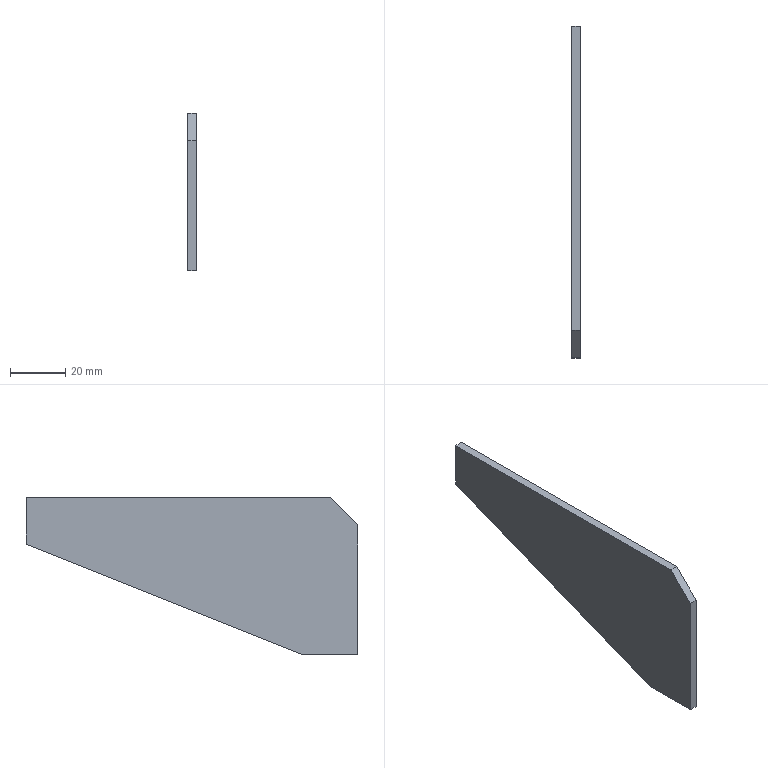Part | STEP file | HL4GZ-1.581.104 (tank support seat rib) | 1 solid | 8 faces | box 3 x 120 x 57 mm | volume 14370 mm3 | plane 8
STEP:
#1=CARTESIAN_POINT('',(0.,0.,0.));
#2=DIRECTION('',(0.,0.,1.));
#3=DIRECTION('',(1.,0.,0.));
#4=AXIS2_PLACEMENT_3D('',#1,#2,#3);
#5=CARTESIAN_POINT('',(1865.,-520.,-328.));
#6=VERTEX_POINT('',#5);
#7=CARTESIAN_POINT('',(1865.,-530.,-338.));
#8=VERTEX_POINT('',#7);
#9=CARTESIAN_POINT('',(1865.,-585.,-393.));
#10=DIRECTION('',(0.,-0.7071,-0.7071));
#11=VECTOR('',#10,1.);
#12=LINE('',#9,#11);
#13=CARTESIAN_POINT('',(1862.,-530.,-338.));
#14=DIRECTION('',(0.,0.7071,-0.7071));
#15=DIRECTION('',(1.,0.,0.));
#16=AXIS2_PLACEMENT_3D('',#13,#14,#15);
#17=PLANE('',#16);
#18=CARTESIAN_POINT('',(3.,77.782));
#19=DIRECTION('',(0.,1.));
#20=VECTOR('',#19,1.);
#21=LINE('',#18,#20);
#22=(GEOMETRIC_REPRESENTATION_CONTEXT(2)PARAMETRIC_REPRESENTATION_CONTEXT()REPRESENTATION_CONTEXT('',''));
#23=DEFINITIONAL_REPRESENTATION('',(#21),#22);
#24=PCURVE('',#17,#23);
#25=CARTESIAN_POINT('',(1865.,-653.,-325.));
#26=DIRECTION('',(1.,0.,0.));
#27=DIRECTION('',(0.,1.,0.));
#28=AXIS2_PLACEMENT_3D('',#25,#26,#27);
#29=PLANE('',#28);
#30=CARTESIAN_POINT('',(68.,-68.));
#31=DIRECTION('',(-0.7071,-0.7071));
#32=VECTOR('',#31,1.);
#33=LINE('',#30,#32);
#34=(GEOMETRIC_REPRESENTATION_CONTEXT(2)PARAMETRIC_REPRESENTATION_CONTEXT()REPRESENTATION_CONTEXT('',''));
#35=DEFINITIONAL_REPRESENTATION('',(#33),#34);
#36=PCURVE('',#29,#35);
#37=SURFACE_CURVE('',#12,(#24,#36),.PCURVE_S1.);
#38=EDGE_CURVE('',#6,#8,#37,.T.);
#39=ORIENTED_EDGE('',*,*,#38,.F.);
#40=CARTESIAN_POINT('',(1862.,-520.,-328.));
#41=VERTEX_POINT('',#40);
#42=CARTESIAN_POINT('',(1863.5,-520.,-328.));
#43=DIRECTION('',(1.,0.,0.));
#44=VECTOR('',#43,1.);
#45=LINE('',#42,#44);
#46=CARTESIAN_POINT('',(1.5,-14.142));
#47=DIRECTION('',(1.,0.));
#48=VECTOR('',#47,1.);
#49=LINE('',#46,#48);
#50=(GEOMETRIC_REPRESENTATION_CONTEXT(2)PARAMETRIC_REPRESENTATION_CONTEXT()REPRESENTATION_CONTEXT('',''));
#51=DEFINITIONAL_REPRESENTATION('',(#49),#50);
#52=PCURVE('',#17,#51);
#53=CARTESIAN_POINT('',(1863.5,-480.,-328.));
#54=DIRECTION('',(0.,0.,1.));
#55=DIRECTION('',(-1.,0.,0.));
#56=AXIS2_PLACEMENT_3D('',#53,#54,#55);
#57=PLANE('',#56);
#58=CARTESIAN_POINT('',(0.,40.));
#59=DIRECTION('',(-1.,0.));
#60=VECTOR('',#59,1.);
#61=LINE('',#58,#60);
#62=(GEOMETRIC_REPRESENTATION_CONTEXT(2)PARAMETRIC_REPRESENTATION_CONTEXT()REPRESENTATION_CONTEXT('',''));
#63=DEFINITIONAL_REPRESENTATION('',(#61),#62);
#64=PCURVE('',#57,#63);
#65=SURFACE_CURVE('',#45,(#52,#64),.PCURVE_S1.);
#66=EDGE_CURVE('',#41,#6,#65,.T.);
#67=ORIENTED_EDGE('',*,*,#66,.F.);
#68=CARTESIAN_POINT('',(1862.,-530.,-338.));
#69=VERTEX_POINT('',#68);
#70=CARTESIAN_POINT('',(1862.,-530.,-338.));
#71=DIRECTION('',(0.,0.7071,0.7071));
#72=VECTOR('',#71,1.);
#73=LINE('',#70,#72);
#74=CARTESIAN_POINT('',(0.,0.));
#75=DIRECTION('',(0.,-1.));
#76=VECTOR('',#75,1.);
#77=LINE('',#74,#76);
#78=(GEOMETRIC_REPRESENTATION_CONTEXT(2)PARAMETRIC_REPRESENTATION_CONTEXT()REPRESENTATION_CONTEXT('',''));
#79=DEFINITIONAL_REPRESENTATION('',(#77),#78);
#80=PCURVE('',#17,#79);
#81=CARTESIAN_POINT('',(1862.,-653.,-325.));
#82=DIRECTION('',(1.,0.,0.));
#83=DIRECTION('',(0.,1.,0.));
#84=AXIS2_PLACEMENT_3D('',#81,#82,#83);
#85=PLANE('',#84);
#86=CARTESIAN_POINT('',(123.,-13.));
#87=DIRECTION('',(0.7071,0.7071));
#88=VECTOR('',#87,1.);
#89=LINE('',#86,#88);
#90=(GEOMETRIC_REPRESENTATION_CONTEXT(2)PARAMETRIC_REPRESENTATION_CONTEXT()REPRESENTATION_CONTEXT('',''));
#91=DEFINITIONAL_REPRESENTATION('',(#89),#90);
#92=PCURVE('',#85,#91);
#93=SURFACE_CURVE('',#73,(#80,#92),.PCURVE_S1.);
#94=EDGE_CURVE('',#69,#41,#93,.T.);
#95=ORIENTED_EDGE('',*,*,#94,.F.);
#96=CARTESIAN_POINT('',(1862.,-530.,-338.));
#97=DIRECTION('',(-1.,0.,0.));
#98=VECTOR('',#97,1.);
#99=LINE('',#96,#98);
#100=CARTESIAN_POINT('',(0.,0.));
#101=DIRECTION('',(-1.,0.));
#102=VECTOR('',#101,1.);
#103=LINE('',#100,#102);
#104=(GEOMETRIC_REPRESENTATION_CONTEXT(2)PARAMETRIC_REPRESENTATION_CONTEXT()REPRESENTATION_CONTEXT('',''));
#105=DEFINITIONAL_REPRESENTATION('',(#103),#104);
#106=PCURVE('',#17,#105);
#107=CARTESIAN_POINT('',(1862.,-530.,-325.));
#108=DIRECTION('',(0.,-1.,0.));
#109=DIRECTION('',(0.,0.,1.));
#110=AXIS2_PLACEMENT_3D('',#107,#108,#109);
#111=PLANE('',#110);
#112=CARTESIAN_POINT('',(-13.,0.));
#113=DIRECTION('',(0.,1.));
#114=VECTOR('',#113,1.);
#115=LINE('',#112,#114);
#116=(GEOMETRIC_REPRESENTATION_CONTEXT(2)PARAMETRIC_REPRESENTATION_CONTEXT()REPRESENTATION_CONTEXT('',''));
#117=DEFINITIONAL_REPRESENTATION('',(#115),#116);
#118=PCURVE('',#111,#117);
#119=SURFACE_CURVE('',#99,(#106,#118),.PCURVE_S1.);
#120=EDGE_CURVE('',#8,#69,#119,.T.);
#121=ORIENTED_EDGE('',*,*,#120,.F.);
#122=EDGE_LOOP('',(#39,#67,#95,#121));
#123=FACE_BOUND('',#122,.T.);
#124=ADVANCED_FACE('',(#123),#17,.F.);
#125=CARTESIAN_POINT('',(1862.,-410.,-328.));
#126=VERTEX_POINT('',#125);
#127=CARTESIAN_POINT('',(1862.,-653.,-328.));
#128=DIRECTION('',(0.,-1.,0.));
#129=VECTOR('',#128,1.);
#130=LINE('',#127,#129);
#131=CARTESIAN_POINT('',(1.5,173.));
#132=DIRECTION('',(0.,1.));
#133=VECTOR('',#132,1.);
#134=LINE('',#131,#133);
#135=(GEOMETRIC_REPRESENTATION_CONTEXT(2)PARAMETRIC_REPRESENTATION_CONTEXT()REPRESENTATION_CONTEXT('',''));
#136=DEFINITIONAL_REPRESENTATION('',(#134),#135);
#137=PCURVE('',#57,#136);
#138=CARTESIAN_POINT('',(0.,-3.));
#139=DIRECTION('',(-1.,0.));
#140=VECTOR('',#139,1.);
#141=LINE('',#138,#140);
#142=(GEOMETRIC_REPRESENTATION_CONTEXT(2)PARAMETRIC_REPRESENTATION_CONTEXT()REPRESENTATION_CONTEXT('',''));
#143=DEFINITIONAL_REPRESENTATION('',(#141),#142);
#144=PCURVE('',#85,#143);
#145=SURFACE_CURVE('',#130,(#137,#144),.PCURVE_S1.);
#146=EDGE_CURVE('',#126,#41,#145,.T.);
#147=ORIENTED_EDGE('',*,*,#146,.T.);
#148=ORIENTED_EDGE('',*,*,#66,.T.);
#149=CARTESIAN_POINT('',(1865.,-410.,-328.));
#150=VERTEX_POINT('',#149);
#151=CARTESIAN_POINT('',(1865.,-653.,-328.));
#152=DIRECTION('',(0.,-1.,0.));
#153=VECTOR('',#152,1.);
#154=LINE('',#151,#153);
#155=CARTESIAN_POINT('',(-1.5,173.));
#156=DIRECTION('',(0.,1.));
#157=VECTOR('',#156,1.);
#158=LINE('',#155,#157);
#159=(GEOMETRIC_REPRESENTATION_CONTEXT(2)PARAMETRIC_REPRESENTATION_CONTEXT()REPRESENTATION_CONTEXT('',''));
#160=DEFINITIONAL_REPRESENTATION('',(#158),#159);
#161=PCURVE('',#57,#160);
#162=CARTESIAN_POINT('',(0.,-3.));
#163=DIRECTION('',(-1.,0.));
#164=VECTOR('',#163,1.);
#165=LINE('',#162,#164);
#166=(GEOMETRIC_REPRESENTATION_CONTEXT(2)PARAMETRIC_REPRESENTATION_CONTEXT()REPRESENTATION_CONTEXT('',''));
#167=DEFINITIONAL_REPRESENTATION('',(#165),#166);
#168=PCURVE('',#29,#167);
#169=SURFACE_CURVE('',#154,(#161,#168),.PCURVE_S1.);
#170=EDGE_CURVE('',#150,#6,#169,.T.);
#171=ORIENTED_EDGE('',*,*,#170,.F.);
#172=CARTESIAN_POINT('',(1862.,-410.,-328.));
#173=DIRECTION('',(1.,0.,0.));
#174=VECTOR('',#173,1.);
#175=LINE('',#172,#174);
#176=CARTESIAN_POINT('',(1.5,-70.));
#177=DIRECTION('',(-1.,0.));
#178=VECTOR('',#177,1.);
#179=LINE('',#176,#178);
#180=(GEOMETRIC_REPRESENTATION_CONTEXT(2)PARAMETRIC_REPRESENTATION_CONTEXT()REPRESENTATION_CONTEXT('',''));
#181=DEFINITIONAL_REPRESENTATION('',(#179),#180);
#182=PCURVE('',#57,#181);
#183=CARTESIAN_POINT('',(1862.,-410.,-325.));
#184=DIRECTION('',(0.,-1.,0.));
#185=DIRECTION('',(0.,0.,1.));
#186=AXIS2_PLACEMENT_3D('',#183,#184,#185);
#187=PLANE('',#186);
#188=CARTESIAN_POINT('',(-3.,0.));
#189=DIRECTION('',(0.,-1.));
#190=VECTOR('',#189,1.);
#191=LINE('',#188,#190);
#192=(GEOMETRIC_REPRESENTATION_CONTEXT(2)PARAMETRIC_REPRESENTATION_CONTEXT()REPRESENTATION_CONTEXT('',''));
#193=DEFINITIONAL_REPRESENTATION('',(#191),#192);
#194=PCURVE('',#187,#193);
#195=SURFACE_CURVE('',#175,(#182,#194),.PCURVE_S1.);
#196=EDGE_CURVE('',#126,#150,#195,.T.);
#197=ORIENTED_EDGE('',*,*,#196,.F.);
#198=EDGE_LOOP('',(#147,#148,#171,#197));
#199=FACE_BOUND('',#198,.T.);
#200=ADVANCED_FACE('',(#199),#57,.T.);
#201=CARTESIAN_POINT('',(1862.,-510.,-385.));
#202=VERTEX_POINT('',#201);
#203=CARTESIAN_POINT('',(1862.,-410.,-345.));
#204=VERTEX_POINT('',#203);
#205=CARTESIAN_POINT('',(1862.,-612.586,-426.034));
#206=DIRECTION('',(0.,0.9285,0.3714));
#207=VECTOR('',#206,1.);
#208=LINE('',#205,#207);
#209=CARTESIAN_POINT('',(1862.,-510.,-385.));
#210=DIRECTION('',(0.,-0.3714,0.9285));
#211=DIRECTION('',(0.,0.9285,0.3714));
#212=AXIS2_PLACEMENT_3D('',#209,#210,#211);
#213=PLANE('',#212);
#214=CARTESIAN_POINT('',(-110.489,0.));
#215=DIRECTION('',(1.,0.));
#216=VECTOR('',#215,1.);
#217=LINE('',#214,#216);
#218=(GEOMETRIC_REPRESENTATION_CONTEXT(2)PARAMETRIC_REPRESENTATION_CONTEXT()REPRESENTATION_CONTEXT('',''));
#219=DEFINITIONAL_REPRESENTATION('',(#217),#218);
#220=PCURVE('',#213,#219);
#221=CARTESIAN_POINT('',(40.414,-101.034));
#222=DIRECTION('',(0.9285,0.3714));
#223=VECTOR('',#222,1.);
#224=LINE('',#221,#223);
#225=(GEOMETRIC_REPRESENTATION_CONTEXT(2)PARAMETRIC_REPRESENTATION_CONTEXT()REPRESENTATION_CONTEXT('',''));
#226=DEFINITIONAL_REPRESENTATION('',(#224),#225);
#227=PCURVE('',#85,#226);
#228=SURFACE_CURVE('',#208,(#220,#227),.PCURVE_S1.);
#229=EDGE_CURVE('',#202,#204,#228,.T.);
#230=ORIENTED_EDGE('',*,*,#229,.T.);
#231=CARTESIAN_POINT('',(1865.,-410.,-345.));
#232=VERTEX_POINT('',#231);
#233=CARTESIAN_POINT('',(1862.,-410.,-345.));
#234=DIRECTION('',(1.,0.,0.));
#235=VECTOR('',#234,1.);
#236=LINE('',#233,#235);
#237=CARTESIAN_POINT('',(107.703,0.));
#238=DIRECTION('',(0.,-1.));
#239=VECTOR('',#238,1.);
#240=LINE('',#237,#239);
#241=(GEOMETRIC_REPRESENTATION_CONTEXT(2)PARAMETRIC_REPRESENTATION_CONTEXT()REPRESENTATION_CONTEXT('',''));
#242=DEFINITIONAL_REPRESENTATION('',(#240),#241);
#243=PCURVE('',#213,#242);
#244=CARTESIAN_POINT('',(-20.,0.));
#245=DIRECTION('',(0.,-1.));
#246=VECTOR('',#245,1.);
#247=LINE('',#244,#246);
#248=(GEOMETRIC_REPRESENTATION_CONTEXT(2)PARAMETRIC_REPRESENTATION_CONTEXT()REPRESENTATION_CONTEXT('',''));
#249=DEFINITIONAL_REPRESENTATION('',(#247),#248);
#250=PCURVE('',#187,#249);
#251=SURFACE_CURVE('',#236,(#243,#250),.PCURVE_S1.);
#252=EDGE_CURVE('',#204,#232,#251,.T.);
#253=ORIENTED_EDGE('',*,*,#252,.T.);
#254=CARTESIAN_POINT('',(1865.,-510.,-385.));
#255=VERTEX_POINT('',#254);
#256=CARTESIAN_POINT('',(1865.,-612.586,-426.034));
#257=DIRECTION('',(0.,0.9285,0.3714));
#258=VECTOR('',#257,1.);
#259=LINE('',#256,#258);
#260=CARTESIAN_POINT('',(-110.489,-3.));
#261=DIRECTION('',(1.,0.));
#262=VECTOR('',#261,1.);
#263=LINE('',#260,#262);
#264=(GEOMETRIC_REPRESENTATION_CONTEXT(2)PARAMETRIC_REPRESENTATION_CONTEXT()REPRESENTATION_CONTEXT('',''));
#265=DEFINITIONAL_REPRESENTATION('',(#263),#264);
#266=PCURVE('',#213,#265);
#267=CARTESIAN_POINT('',(40.414,-101.034));
#268=DIRECTION('',(0.9285,0.3714));
#269=VECTOR('',#268,1.);
#270=LINE('',#267,#269);
#271=(GEOMETRIC_REPRESENTATION_CONTEXT(2)PARAMETRIC_REPRESENTATION_CONTEXT()REPRESENTATION_CONTEXT('',''));
#272=DEFINITIONAL_REPRESENTATION('',(#270),#271);
#273=PCURVE('',#29,#272);
#274=SURFACE_CURVE('',#259,(#266,#273),.PCURVE_S1.);
#275=EDGE_CURVE('',#255,#232,#274,.T.);
#276=ORIENTED_EDGE('',*,*,#275,.F.);
#277=CARTESIAN_POINT('',(1862.,-510.,-385.));
#278=DIRECTION('',(1.,0.,0.));
#279=VECTOR('',#278,1.);
#280=LINE('',#277,#279);
#281=CARTESIAN_POINT('',(0.,0.));
#282=DIRECTION('',(0.,-1.));
#283=VECTOR('',#282,1.);
#284=LINE('',#281,#283);
#285=(GEOMETRIC_REPRESENTATION_CONTEXT(2)PARAMETRIC_REPRESENTATION_CONTEXT()REPRESENTATION_CONTEXT('',''));
#286=DEFINITIONAL_REPRESENTATION('',(#284),#285);
#287=PCURVE('',#213,#286);
#288=CARTESIAN_POINT('',(1862.,-430.,-385.));
#289=DIRECTION('',(0.,0.,1.));
#290=DIRECTION('',(0.,1.,0.));
#291=AXIS2_PLACEMENT_3D('',#288,#289,#290);
#292=PLANE('',#291);
#293=CARTESIAN_POINT('',(-80.,0.));
#294=DIRECTION('',(0.,-1.));
#295=VECTOR('',#294,1.);
#296=LINE('',#293,#295);
#297=(GEOMETRIC_REPRESENTATION_CONTEXT(2)PARAMETRIC_REPRESENTATION_CONTEXT()REPRESENTATION_CONTEXT('',''));
#298=DEFINITIONAL_REPRESENTATION('',(#296),#297);
#299=PCURVE('',#292,#298);
#300=SURFACE_CURVE('',#280,(#287,#299),.PCURVE_S1.);
#301=EDGE_CURVE('',#202,#255,#300,.T.);
#302=ORIENTED_EDGE('',*,*,#301,.F.);
#303=EDGE_LOOP('',(#230,#253,#276,#302));
#304=FACE_BOUND('',#303,.T.);
#305=ADVANCED_FACE('',(#304),#213,.F.);
#306=CARTESIAN_POINT('',(1862.,-530.,-385.));
#307=VERTEX_POINT('',#306);
#308=CARTESIAN_POINT('',(1865.,-530.,-385.));
#309=VERTEX_POINT('',#308);
#310=CARTESIAN_POINT('',(1862.,-530.,-385.));
#311=DIRECTION('',(1.,0.,0.));
#312=VECTOR('',#311,1.);
#313=LINE('',#310,#312);
#314=CARTESIAN_POINT('',(-100.,0.));
#315=DIRECTION('',(0.,-1.));
#316=VECTOR('',#315,1.);
#317=LINE('',#314,#316);
#318=(GEOMETRIC_REPRESENTATION_CONTEXT(2)PARAMETRIC_REPRESENTATION_CONTEXT()REPRESENTATION_CONTEXT('',''));
#319=DEFINITIONAL_REPRESENTATION('',(#317),#318);
#320=PCURVE('',#292,#319);
#321=CARTESIAN_POINT('',(-60.,0.));
#322=DIRECTION('',(0.,-1.));
#323=VECTOR('',#322,1.);
#324=LINE('',#321,#323);
#325=(GEOMETRIC_REPRESENTATION_CONTEXT(2)PARAMETRIC_REPRESENTATION_CONTEXT()REPRESENTATION_CONTEXT('',''));
#326=DEFINITIONAL_REPRESENTATION('',(#324),#325);
#327=PCURVE('',#111,#326);
#328=SURFACE_CURVE('',#313,(#320,#327),.PCURVE_S1.);
#329=EDGE_CURVE('',#307,#309,#328,.T.);
#330=ORIENTED_EDGE('',*,*,#329,.F.);
#331=CARTESIAN_POINT('',(1862.,-430.,-385.));
#332=DIRECTION('',(0.,-1.,0.));
#333=VECTOR('',#332,1.);
#334=LINE('',#331,#333);
#335=CARTESIAN_POINT('',(0.,0.));
#336=DIRECTION('',(-1.,0.));
#337=VECTOR('',#336,1.);
#338=LINE('',#335,#337);
#339=(GEOMETRIC_REPRESENTATION_CONTEXT(2)PARAMETRIC_REPRESENTATION_CONTEXT()REPRESENTATION_CONTEXT('',''));
#340=DEFINITIONAL_REPRESENTATION('',(#338),#339);
#341=PCURVE('',#292,#340);
#342=CARTESIAN_POINT('',(223.,-60.));
#343=DIRECTION('',(-1.,0.));
#344=VECTOR('',#343,1.);
#345=LINE('',#342,#344);
#346=(GEOMETRIC_REPRESENTATION_CONTEXT(2)PARAMETRIC_REPRESENTATION_CONTEXT()REPRESENTATION_CONTEXT('',''));
#347=DEFINITIONAL_REPRESENTATION('',(#345),#346);
#348=PCURVE('',#85,#347);
#349=SURFACE_CURVE('',#334,(#341,#348),.PCURVE_S1.);
#350=EDGE_CURVE('',#202,#307,#349,.T.);
#351=ORIENTED_EDGE('',*,*,#350,.F.);
#352=ORIENTED_EDGE('',*,*,#301,.T.);
#353=CARTESIAN_POINT('',(1865.,-653.,-385.));
#354=DIRECTION('',(0.,-1.,0.));
#355=VECTOR('',#354,1.);
#356=LINE('',#353,#355);
#357=CARTESIAN_POINT('',(-223.,-3.));
#358=DIRECTION('',(-1.,0.));
#359=VECTOR('',#358,1.);
#360=LINE('',#357,#359);
#361=(GEOMETRIC_REPRESENTATION_CONTEXT(2)PARAMETRIC_REPRESENTATION_CONTEXT()REPRESENTATION_CONTEXT('',''));
#362=DEFINITIONAL_REPRESENTATION('',(#360),#361);
#363=PCURVE('',#292,#362);
#364=CARTESIAN_POINT('',(0.,-60.));
#365=DIRECTION('',(-1.,0.));
#366=VECTOR('',#365,1.);
#367=LINE('',#364,#366);
#368=(GEOMETRIC_REPRESENTATION_CONTEXT(2)PARAMETRIC_REPRESENTATION_CONTEXT()REPRESENTATION_CONTEXT('',''));
#369=DEFINITIONAL_REPRESENTATION('',(#367),#368);
#370=PCURVE('',#29,#369);
#371=SURFACE_CURVE('',#356,(#363,#370),.PCURVE_S1.);
#372=EDGE_CURVE('',#255,#309,#371,.T.);
#373=ORIENTED_EDGE('',*,*,#372,.T.);
#374=EDGE_LOOP('',(#330,#351,#352,#373));
#375=FACE_BOUND('',#374,.T.);
#376=ADVANCED_FACE('',(#375),#292,.F.);
#377=CARTESIAN_POINT('',(1862.,-530.,-325.));
#378=DIRECTION('',(0.,0.,-1.));
#379=VECTOR('',#378,1.);
#380=LINE('',#377,#379);
#381=CARTESIAN_POINT('',(123.,0.));
#382=DIRECTION('',(0.,-1.));
#383=VECTOR('',#382,1.);
#384=LINE('',#381,#383);
#385=(GEOMETRIC_REPRESENTATION_CONTEXT(2)PARAMETRIC_REPRESENTATION_CONTEXT()REPRESENTATION_CONTEXT('',''));
#386=DEFINITIONAL_REPRESENTATION('',(#384),#385);
#387=PCURVE('',#85,#386);
#388=CARTESIAN_POINT('',(0.,0.));
#389=DIRECTION('',(-1.,0.));
#390=VECTOR('',#389,1.);
#391=LINE('',#388,#390);
#392=(GEOMETRIC_REPRESENTATION_CONTEXT(2)PARAMETRIC_REPRESENTATION_CONTEXT()REPRESENTATION_CONTEXT('',''));
#393=DEFINITIONAL_REPRESENTATION('',(#391),#392);
#394=PCURVE('',#111,#393);
#395=SURFACE_CURVE('',#380,(#387,#394),.PCURVE_S1.);
#396=EDGE_CURVE('',#69,#307,#395,.T.);
#397=ORIENTED_EDGE('',*,*,#396,.F.);
#398=ORIENTED_EDGE('',*,*,#94,.T.);
#399=ORIENTED_EDGE('',*,*,#146,.F.);
#400=CARTESIAN_POINT('',(1862.,-410.,-325.));
#401=DIRECTION('',(0.,0.,-1.));
#402=VECTOR('',#401,1.);
#403=LINE('',#400,#402);
#404=CARTESIAN_POINT('',(243.,0.));
#405=DIRECTION('',(0.,-1.));
#406=VECTOR('',#405,1.);
#407=LINE('',#404,#406);
#408=(GEOMETRIC_REPRESENTATION_CONTEXT(2)PARAMETRIC_REPRESENTATION_CONTEXT()REPRESENTATION_CONTEXT('',''));
#409=DEFINITIONAL_REPRESENTATION('',(#407),#408);
#410=PCURVE('',#85,#409);
#411=CARTESIAN_POINT('',(0.,0.));
#412=DIRECTION('',(-1.,0.));
#413=VECTOR('',#412,1.);
#414=LINE('',#411,#413);
#415=(GEOMETRIC_REPRESENTATION_CONTEXT(2)PARAMETRIC_REPRESENTATION_CONTEXT()REPRESENTATION_CONTEXT('',''));
#416=DEFINITIONAL_REPRESENTATION('',(#414),#415);
#417=PCURVE('',#187,#416);
#418=SURFACE_CURVE('',#403,(#410,#417),.PCURVE_S1.);
#419=EDGE_CURVE('',#126,#204,#418,.T.);
#420=ORIENTED_EDGE('',*,*,#419,.T.);
#421=ORIENTED_EDGE('',*,*,#229,.F.);
#422=ORIENTED_EDGE('',*,*,#350,.T.);
#423=EDGE_LOOP('',(#397,#398,#399,#420,#421,#422));
#424=FACE_BOUND('',#423,.T.);
#425=ADVANCED_FACE('',(#424),#85,.F.);
#426=ORIENTED_EDGE('',*,*,#170,.T.);
#427=ORIENTED_EDGE('',*,*,#38,.T.);
#428=CARTESIAN_POINT('',(1865.,-530.,-325.));
#429=DIRECTION('',(0.,0.,-1.));
#430=VECTOR('',#429,1.);
#431=LINE('',#428,#430);
#432=CARTESIAN_POINT('',(123.,0.));
#433=DIRECTION('',(0.,-1.));
#434=VECTOR('',#433,1.);
#435=LINE('',#432,#434);
#436=(GEOMETRIC_REPRESENTATION_CONTEXT(2)PARAMETRIC_REPRESENTATION_CONTEXT()REPRESENTATION_CONTEXT('',''));
#437=DEFINITIONAL_REPRESENTATION('',(#435),#436);
#438=PCURVE('',#29,#437);
#439=CARTESIAN_POINT('',(0.,-3.));
#440=DIRECTION('',(-1.,0.));
#441=VECTOR('',#440,1.);
#442=LINE('',#439,#441);
#443=(GEOMETRIC_REPRESENTATION_CONTEXT(2)PARAMETRIC_REPRESENTATION_CONTEXT()REPRESENTATION_CONTEXT('',''));
#444=DEFINITIONAL_REPRESENTATION('',(#442),#443);
#445=PCURVE('',#111,#444);
#446=SURFACE_CURVE('',#431,(#438,#445),.PCURVE_S1.);
#447=EDGE_CURVE('',#8,#309,#446,.T.);
#448=ORIENTED_EDGE('',*,*,#447,.T.);
#449=ORIENTED_EDGE('',*,*,#372,.F.);
#450=ORIENTED_EDGE('',*,*,#275,.T.);
#451=CARTESIAN_POINT('',(1865.,-410.,-325.));
#452=DIRECTION('',(0.,0.,-1.));
#453=VECTOR('',#452,1.);
#454=LINE('',#451,#453);
#455=CARTESIAN_POINT('',(243.,0.));
#456=DIRECTION('',(0.,-1.));
#457=VECTOR('',#456,1.);
#458=LINE('',#455,#457);
#459=(GEOMETRIC_REPRESENTATION_CONTEXT(2)PARAMETRIC_REPRESENTATION_CONTEXT()REPRESENTATION_CONTEXT('',''));
#460=DEFINITIONAL_REPRESENTATION('',(#458),#459);
#461=PCURVE('',#29,#460);
#462=CARTESIAN_POINT('',(0.,-3.));
#463=DIRECTION('',(-1.,0.));
#464=VECTOR('',#463,1.);
#465=LINE('',#462,#464);
#466=(GEOMETRIC_REPRESENTATION_CONTEXT(2)PARAMETRIC_REPRESENTATION_CONTEXT()REPRESENTATION_CONTEXT('',''));
#467=DEFINITIONAL_REPRESENTATION('',(#465),#466);
#468=PCURVE('',#187,#467);
#469=SURFACE_CURVE('',#454,(#461,#468),.PCURVE_S1.);
#470=EDGE_CURVE('',#150,#232,#469,.T.);
#471=ORIENTED_EDGE('',*,*,#470,.F.);
#472=EDGE_LOOP('',(#426,#427,#448,#449,#450,#471));
#473=FACE_BOUND('',#472,.T.);
#474=ADVANCED_FACE('',(#473),#29,.T.);
#475=ORIENTED_EDGE('',*,*,#447,.F.);
#476=ORIENTED_EDGE('',*,*,#120,.T.);
#477=ORIENTED_EDGE('',*,*,#396,.T.);
#478=ORIENTED_EDGE('',*,*,#329,.T.);
#479=EDGE_LOOP('',(#475,#476,#477,#478));
#480=FACE_BOUND('',#479,.T.);
#481=ADVANCED_FACE('',(#480),#111,.T.);
#482=ORIENTED_EDGE('',*,*,#419,.F.);
#483=ORIENTED_EDGE('',*,*,#196,.T.);
#484=ORIENTED_EDGE('',*,*,#470,.T.);
#485=ORIENTED_EDGE('',*,*,#252,.F.);
#486=EDGE_LOOP('',(#482,#483,#484,#485));
#487=FACE_BOUND('',#486,.T.);
#488=ADVANCED_FACE('',(#487),#187,.F.);
#489=CLOSED_SHELL('',(#124,#200,#305,#376,#425,#474,#481,#488));
#490=MANIFOLD_SOLID_BREP('',#489);
#491=(LENGTH_UNIT()NAMED_UNIT(*)SI_UNIT(.MILLI.,.METRE.));
#492=UNCERTAINTY_MEASURE_WITH_UNIT(LENGTH_MEASURE(0.0000001),#491,'','');
#493=(NAMED_UNIT(*)PLANE_ANGLE_UNIT()SI_UNIT($,.RADIAN.));
#494=(NAMED_UNIT(*)SI_UNIT($,.STERADIAN.)SOLID_ANGLE_UNIT());
#495=(GEOMETRIC_REPRESENTATION_CONTEXT(3)GLOBAL_UNCERTAINTY_ASSIGNED_CONTEXT((#492))GLOBAL_UNIT_ASSIGNED_CONTEXT((#491,#493,#494))REPRESENTATION_CONTEXT('',''));
#496=ADVANCED_BREP_SHAPE_REPRESENTATION('',(#4,#490),#495);